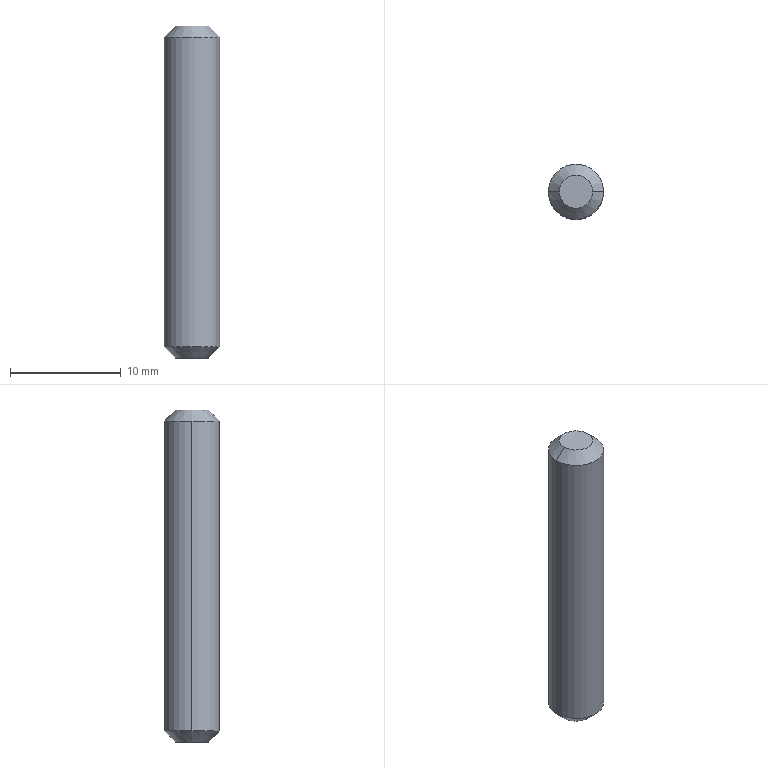Part | SolidWorks | features Chamfer 1, Extrusion 1 | 1 solid | 8 faces | box 5 x 5 x 30 mm | volume 575.435 mm3 | cone 4 | cylinder 2 | plane 2 | commonest cylinder face diameters 5 x2
STEP:
#1=CARTESIAN_POINT('',(1.5,0.,30.));
#2=VERTEX_POINT('',#1);
#3=CARTESIAN_POINT('',(-1.5,0.,30.));
#4=VERTEX_POINT('',#3);
#5=CARTESIAN_POINT('',(0.,0.,30.));
#6=DIRECTION('',(0.,0.,1.));
#7=DIRECTION('',(1.,0.,0.));
#8=AXIS2_PLACEMENT_3D('',#5,#6,#7);
#9=CIRCLE('',#8,1.5);
#10=EDGE_CURVE('',#2,#4,#9,.T.);
#11=ORIENTED_EDGE('',*,*,#10,.F.);
#12=CARTESIAN_POINT('',(2.5,0.,29.));
#13=VERTEX_POINT('',#12);
#14=CARTESIAN_POINT('',(1.5,0.,30.));
#15=DIRECTION('',(0.7071,0.,-0.7071));
#16=VECTOR('',#15,1000.);
#17=LINE('',#14,#16);
#18=EDGE_CURVE('',#2,#13,#17,.T.);
#19=ORIENTED_EDGE('',*,*,#18,.T.);
#20=CARTESIAN_POINT('',(-2.5,0.,29.));
#21=VERTEX_POINT('',#20);
#22=CARTESIAN_POINT('',(0.,0.,29.));
#23=DIRECTION('',(0.,0.,-1.));
#24=DIRECTION('',(1.,0.,0.));
#25=AXIS2_PLACEMENT_3D('',#22,#23,#24);
#26=CIRCLE('',#25,2.5);
#27=EDGE_CURVE('',#21,#13,#26,.T.);
#28=ORIENTED_EDGE('',*,*,#27,.F.);
#29=CARTESIAN_POINT('',(-1.5,0.,30.));
#30=DIRECTION('',(-0.7071,0.,-0.7071));
#31=VECTOR('',#30,1000.);
#32=LINE('',#29,#31);
#33=EDGE_CURVE('',#4,#21,#32,.T.);
#34=ORIENTED_EDGE('',*,*,#33,.F.);
#35=EDGE_LOOP('',(#11,#19,#28,#34));
#36=FACE_OUTER_BOUND('',#35,.T.);
#37=CARTESIAN_POINT('',(0.,0.,30.));
#38=DIRECTION('',(0.,0.,-1.));
#39=DIRECTION('',(-1.,0.,0.));
#40=AXIS2_PLACEMENT_3D('',#37,#38,#39);
#41=CONICAL_SURFACE('',#40,1.5,0.7854);
#42=ADVANCED_FACE('',(#36),#41,.T.);
#43=CARTESIAN_POINT('',(-1.5,0.,0.));
#44=VERTEX_POINT('',#43);
#45=CARTESIAN_POINT('',(1.5,0.,0.));
#46=VERTEX_POINT('',#45);
#47=CARTESIAN_POINT('',(0.,0.,0.));
#48=DIRECTION('',(0.,0.,-1.));
#49=DIRECTION('',(1.,0.,0.));
#50=AXIS2_PLACEMENT_3D('',#47,#48,#49);
#51=CIRCLE('',#50,1.5);
#52=EDGE_CURVE('',#44,#46,#51,.T.);
#53=ORIENTED_EDGE('',*,*,#52,.F.);
#54=CARTESIAN_POINT('',(-2.5,0.,1.));
#55=VERTEX_POINT('',#54);
#56=CARTESIAN_POINT('',(-2.5,0.,1.));
#57=DIRECTION('',(-0.7071,0.,0.7071));
#58=VECTOR('',#57,1000.);
#59=LINE('',#56,#58);
#60=EDGE_CURVE('',#44,#55,#59,.T.);
#61=ORIENTED_EDGE('',*,*,#60,.T.);
#62=CARTESIAN_POINT('',(2.5,0.,1.));
#63=VERTEX_POINT('',#62);
#64=CARTESIAN_POINT('',(0.,0.,1.));
#65=DIRECTION('',(0.,0.,1.));
#66=DIRECTION('',(1.,0.,0.));
#67=AXIS2_PLACEMENT_3D('',#64,#65,#66);
#68=CIRCLE('',#67,2.5);
#69=EDGE_CURVE('',#63,#55,#68,.T.);
#70=ORIENTED_EDGE('',*,*,#69,.F.);
#71=CARTESIAN_POINT('',(2.5,0.,1.));
#72=DIRECTION('',(0.7071,0.,0.7071));
#73=VECTOR('',#72,1000.);
#74=LINE('',#71,#73);
#75=EDGE_CURVE('',#46,#63,#74,.T.);
#76=ORIENTED_EDGE('',*,*,#75,.F.);
#77=EDGE_LOOP('',(#53,#61,#70,#76));
#78=FACE_OUTER_BOUND('',#77,.T.);
#79=CARTESIAN_POINT('',(0.,0.,1.));
#80=DIRECTION('',(0.,0.,1.));
#81=DIRECTION('',(1.,0.,0.));
#82=AXIS2_PLACEMENT_3D('',#79,#80,#81);
#83=CONICAL_SURFACE('',#82,2.5,0.7854);
#84=ADVANCED_FACE('',(#78),#83,.T.);
#85=ORIENTED_EDGE('',*,*,#27,.T.);
#86=CARTESIAN_POINT('',(2.5,0.,30.));
#87=DIRECTION('',(0.,0.,-1.));
#88=VECTOR('',#87,1000.);
#89=LINE('',#86,#88);
#90=EDGE_CURVE('',#13,#63,#89,.T.);
#91=ORIENTED_EDGE('',*,*,#90,.T.);
#92=ORIENTED_EDGE('',*,*,#69,.T.);
#93=CARTESIAN_POINT('',(-2.5,0.,30.));
#94=DIRECTION('',(0.,0.,-1.));
#95=VECTOR('',#94,1000.);
#96=LINE('',#93,#95);
#97=EDGE_CURVE('',#21,#55,#96,.T.);
#98=ORIENTED_EDGE('',*,*,#97,.F.);
#99=EDGE_LOOP('',(#85,#91,#92,#98));
#100=FACE_OUTER_BOUND('',#99,.T.);
#101=CARTESIAN_POINT('',(0.,0.,30.));
#102=DIRECTION('',(0.,0.,-1.));
#103=DIRECTION('',(-1.,0.,0.));
#104=AXIS2_PLACEMENT_3D('',#101,#102,#103);
#105=CYLINDRICAL_SURFACE('',#104,2.5);
#106=ADVANCED_FACE('',(#100),#105,.T.);
#107=ORIENTED_EDGE('',*,*,#90,.F.);
#108=CARTESIAN_POINT('',(0.,0.,29.));
#109=DIRECTION('',(0.,0.,-1.));
#110=DIRECTION('',(1.,0.,0.));
#111=AXIS2_PLACEMENT_3D('',#108,#109,#110);
#112=CIRCLE('',#111,2.5);
#113=EDGE_CURVE('',#13,#21,#112,.T.);
#114=ORIENTED_EDGE('',*,*,#113,.T.);
#115=ORIENTED_EDGE('',*,*,#97,.T.);
#116=CARTESIAN_POINT('',(0.,0.,1.));
#117=DIRECTION('',(0.,0.,1.));
#118=DIRECTION('',(1.,0.,0.));
#119=AXIS2_PLACEMENT_3D('',#116,#117,#118);
#120=CIRCLE('',#119,2.5);
#121=EDGE_CURVE('',#55,#63,#120,.T.);
#122=ORIENTED_EDGE('',*,*,#121,.T.);
#123=EDGE_LOOP('',(#107,#114,#115,#122));
#124=FACE_OUTER_BOUND('',#123,.T.);
#125=CARTESIAN_POINT('',(0.,0.,30.));
#126=DIRECTION('',(0.,0.,-1.));
#127=DIRECTION('',(-1.,0.,0.));
#128=AXIS2_PLACEMENT_3D('',#125,#126,#127);
#129=CYLINDRICAL_SURFACE('',#128,2.5);
#130=ADVANCED_FACE('',(#124),#129,.T.);
#131=CARTESIAN_POINT('',(0.,0.,30.));
#132=DIRECTION('',(0.,0.,1.));
#133=DIRECTION('',(1.,0.,0.));
#134=AXIS2_PLACEMENT_3D('',#131,#132,#133);
#135=CIRCLE('',#134,1.5);
#136=EDGE_CURVE('',#4,#2,#135,.T.);
#137=ORIENTED_EDGE('',*,*,#136,.T.);
#138=ORIENTED_EDGE('',*,*,#10,.T.);
#139=EDGE_LOOP('',(#137,#138));
#140=FACE_OUTER_BOUND('',#139,.T.);
#141=CARTESIAN_POINT('',(0.,0.,30.));
#142=DIRECTION('',(0.,0.,1.));
#143=DIRECTION('',(1.,0.,0.));
#144=AXIS2_PLACEMENT_3D('',#141,#142,#143);
#145=PLANE('',#144);
#146=ADVANCED_FACE('',(#140),#145,.T.);
#147=CARTESIAN_POINT('',(0.,0.,0.));
#148=DIRECTION('',(0.,0.,-1.));
#149=DIRECTION('',(1.,0.,0.));
#150=AXIS2_PLACEMENT_3D('',#147,#148,#149);
#151=CIRCLE('',#150,1.5);
#152=EDGE_CURVE('',#46,#44,#151,.T.);
#153=ORIENTED_EDGE('',*,*,#152,.T.);
#154=ORIENTED_EDGE('',*,*,#52,.T.);
#155=EDGE_LOOP('',(#153,#154));
#156=FACE_OUTER_BOUND('',#155,.T.);
#157=CARTESIAN_POINT('',(0.,0.,0.));
#158=DIRECTION('',(0.,0.,1.));
#159=DIRECTION('',(1.,0.,0.));
#160=AXIS2_PLACEMENT_3D('',#157,#158,#159);
#161=PLANE('',#160);
#162=ADVANCED_FACE('',(#156),#161,.F.);
#163=ORIENTED_EDGE('',*,*,#60,.F.);
#164=ORIENTED_EDGE('',*,*,#152,.F.);
#165=ORIENTED_EDGE('',*,*,#75,.T.);
#166=ORIENTED_EDGE('',*,*,#121,.F.);
#167=EDGE_LOOP('',(#163,#164,#165,#166));
#168=FACE_OUTER_BOUND('',#167,.T.);
#169=CARTESIAN_POINT('',(0.,0.,1.));
#170=DIRECTION('',(0.,0.,1.));
#171=DIRECTION('',(1.,0.,0.));
#172=AXIS2_PLACEMENT_3D('',#169,#170,#171);
#173=CONICAL_SURFACE('',#172,2.5,0.7854);
#174=ADVANCED_FACE('',(#168),#173,.T.);
#175=ORIENTED_EDGE('',*,*,#18,.F.);
#176=ORIENTED_EDGE('',*,*,#136,.F.);
#177=ORIENTED_EDGE('',*,*,#33,.T.);
#178=ORIENTED_EDGE('',*,*,#113,.F.);
#179=EDGE_LOOP('',(#175,#176,#177,#178));
#180=FACE_OUTER_BOUND('',#179,.T.);
#181=CARTESIAN_POINT('',(0.,0.,30.));
#182=DIRECTION('',(0.,0.,-1.));
#183=DIRECTION('',(-1.,0.,0.));
#184=AXIS2_PLACEMENT_3D('',#181,#182,#183);
#185=CONICAL_SURFACE('',#184,1.5,0.7854);
#186=ADVANCED_FACE('',(#180),#185,.T.);
#187=CLOSED_SHELL('',(#42,#84,#106,#130,#146,#162,#174,#186));
#188=MANIFOLD_SOLID_BREP('',#187);
#189=CARTESIAN_POINT('',(0.,0.,0.));
#190=DIRECTION('',(0.,0.,1.));
#191=DIRECTION('',(1.,0.,0.));
#192=AXIS2_PLACEMENT_3D('',#189,#190,#191);
#193=(LENGTH_UNIT()NAMED_UNIT(*)SI_UNIT(.MILLI.,.METRE.));
#194=UNCERTAINTY_MEASURE_WITH_UNIT(LENGTH_MEASURE(0.00001),#193,'','');
#195=(NAMED_UNIT(*)PLANE_ANGLE_UNIT()SI_UNIT($,.RADIAN.));
#196=(NAMED_UNIT(*)SI_UNIT($,.STERADIAN.)SOLID_ANGLE_UNIT());
#197=(GEOMETRIC_REPRESENTATION_CONTEXT(3)GLOBAL_UNCERTAINTY_ASSIGNED_CONTEXT((#194))GLOBAL_UNIT_ASSIGNED_CONTEXT((#193,#195,#196))REPRESENTATION_CONTEXT('',''));
#198=ADVANCED_BREP_SHAPE_REPRESENTATION('',(#188,#192),#197);